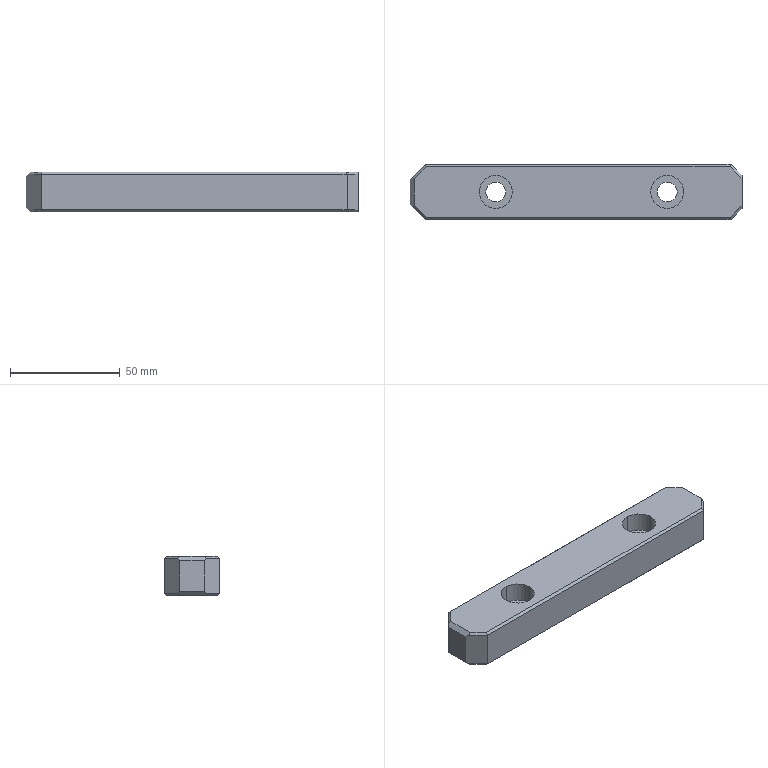Part | Creo | 1 solid | 34 faces | box 151 x 25 x 18 mm | volume 61935 mm3 | plane 26 | cylinder 8 | commonest cylinder face diameters 9 x4 15 x4
STEP:
#1=CARTESIAN_POINT('',(-121.,7.495,-46.5));
#2=VERTEX_POINT('',#1);
#3=CARTESIAN_POINT('',(-121.,7.495,-62.5));
#4=VERTEX_POINT('',#3);
#5=CARTESIAN_POINT('',(-121.,7.495,-46.5));
#6=DIRECTION('',(0.,0.,-1.));
#7=VECTOR('',#6,16.);
#8=LINE('',#5,#7);
#9=EDGE_CURVE('',#2,#4,#8,.T.);
#10=ORIENTED_EDGE('',*,*,#9,.T.);
#11=CARTESIAN_POINT('',(-121.,6.081,-63.5));
#12=VERTEX_POINT('',#11);
#13=CARTESIAN_POINT('',(-121.,6.081,-63.5));
#14=DIRECTION('',(0.,0.8165,0.5774));
#15=VECTOR('',#14,1.732);
#16=LINE('',#13,#15);
#17=EDGE_CURVE('',#12,#4,#16,.T.);
#18=ORIENTED_EDGE('',*,*,#17,.F.);
#19=CARTESIAN_POINT('',(-121.,-6.09,-63.5));
#20=VERTEX_POINT('',#19);
#21=CARTESIAN_POINT('',(-121.,6.081,-63.5));
#22=DIRECTION('',(0.,-1.,0.));
#23=VECTOR('',#22,12.172);
#24=LINE('',#21,#23);
#25=EDGE_CURVE('',#12,#20,#24,.T.);
#26=ORIENTED_EDGE('',*,*,#25,.T.);
#27=CARTESIAN_POINT('',(-121.,-7.505,-62.5));
#28=VERTEX_POINT('',#27);
#29=CARTESIAN_POINT('',(-121.,-7.505,-62.5));
#30=DIRECTION('',(0.,0.8165,-0.5774));
#31=VECTOR('',#30,1.732);
#32=LINE('',#29,#31);
#33=EDGE_CURVE('',#28,#20,#32,.T.);
#34=ORIENTED_EDGE('',*,*,#33,.F.);
#35=CARTESIAN_POINT('',(-121.,-7.505,-46.5));
#36=VERTEX_POINT('',#35);
#37=CARTESIAN_POINT('',(-121.,-7.505,-62.5));
#38=DIRECTION('',(0.,0.,1.));
#39=VECTOR('',#38,16.);
#40=LINE('',#37,#39);
#41=EDGE_CURVE('',#28,#36,#40,.T.);
#42=ORIENTED_EDGE('',*,*,#41,.T.);
#43=CARTESIAN_POINT('',(-121.,-6.09,-45.5));
#44=VERTEX_POINT('',#43);
#45=CARTESIAN_POINT('',(-121.,-6.09,-45.5));
#46=DIRECTION('',(0.,-0.8165,-0.5774));
#47=VECTOR('',#46,1.732);
#48=LINE('',#45,#47);
#49=EDGE_CURVE('',#44,#36,#48,.T.);
#50=ORIENTED_EDGE('',*,*,#49,.F.);
#51=CARTESIAN_POINT('',(-121.,6.081,-45.5));
#52=VERTEX_POINT('',#51);
#53=CARTESIAN_POINT('',(-121.,-6.09,-45.5));
#54=DIRECTION('',(0.,1.,0.));
#55=VECTOR('',#54,12.172);
#56=LINE('',#53,#55);
#57=EDGE_CURVE('',#44,#52,#56,.T.);
#58=ORIENTED_EDGE('',*,*,#57,.T.);
#59=CARTESIAN_POINT('',(-121.,7.495,-46.5));
#60=DIRECTION('',(0.,-0.8165,0.5774));
#61=VECTOR('',#60,1.732);
#62=LINE('',#59,#61);
#63=EDGE_CURVE('',#2,#52,#62,.T.);
#64=ORIENTED_EDGE('',*,*,#63,.F.);
#65=EDGE_LOOP('',(#10,#18,#26,#34,#42,#50,#58,#64));
#66=FACE_OUTER_BOUND('',#65,.F.);
#67=CARTESIAN_POINT('',(-121.,209.995,-11.));
#68=DIRECTION('',(-1.,0.,0.));
#69=DIRECTION('',(0.,-1.,0.));
#70=AXIS2_PLACEMENT_3D('',#67,#68,#69);
#71=PLANE('',#70);
#72=ADVANCED_FACE('',(#66),#71,.F.);
#73=CARTESIAN_POINT('',(-126.,12.495,-46.5));
#74=VERTEX_POINT('',#73);
#75=CARTESIAN_POINT('',(-126.,12.495,-62.5));
#76=VERTEX_POINT('',#75);
#77=CARTESIAN_POINT('',(-126.,12.495,-46.5));
#78=DIRECTION('',(0.,0.,-1.));
#79=VECTOR('',#78,16.);
#80=LINE('',#77,#79);
#81=EDGE_CURVE('',#74,#76,#80,.T.);
#82=ORIENTED_EDGE('',*,*,#81,.T.);
#83=CARTESIAN_POINT('',(-121.,7.495,-62.5));
#84=DIRECTION('',(-0.7071,0.7071,0.));
#85=VECTOR('',#84,7.071);
#86=LINE('',#83,#85);
#87=EDGE_CURVE('',#4,#76,#86,.T.);
#88=ORIENTED_EDGE('',*,*,#87,.F.);
#89=ORIENTED_EDGE('',*,*,#9,.F.);
#90=CARTESIAN_POINT('',(-121.,7.495,-46.5));
#91=DIRECTION('',(-0.7071,0.7071,0.));
#92=VECTOR('',#91,7.071);
#93=LINE('',#90,#92);
#94=EDGE_CURVE('',#2,#74,#93,.T.);
#95=ORIENTED_EDGE('',*,*,#94,.T.);
#96=EDGE_LOOP('',(#82,#88,#89,#95));
#97=FACE_OUTER_BOUND('',#96,.F.);
#98=CARTESIAN_POINT('',(-123.,9.495,-54.5));
#99=DIRECTION('',(0.7071,0.7071,0.));
#100=DIRECTION('',(0.,0.,-1.));
#101=AXIS2_PLACEMENT_3D('',#98,#99,#100);
#102=PLANE('',#101);
#103=ADVANCED_FACE('',(#97),#102,.T.);
#104=CARTESIAN_POINT('',(-265.,12.495,-62.5));
#105=VERTEX_POINT('',#104);
#106=CARTESIAN_POINT('',(-265.,12.495,-46.5));
#107=VERTEX_POINT('',#106);
#108=CARTESIAN_POINT('',(-265.,12.495,-62.5));
#109=DIRECTION('',(0.,0.,1.));
#110=VECTOR('',#109,16.);
#111=LINE('',#108,#110);
#112=EDGE_CURVE('',#105,#107,#111,.T.);
#113=ORIENTED_EDGE('',*,*,#112,.F.);
#114=CARTESIAN_POINT('',(-126.,12.495,-62.5));
#115=DIRECTION('',(-1.,0.,0.));
#116=VECTOR('',#115,139.);
#117=LINE('',#114,#116);
#118=EDGE_CURVE('',#76,#105,#117,.T.);
#119=ORIENTED_EDGE('',*,*,#118,.F.);
#120=ORIENTED_EDGE('',*,*,#81,.F.);
#121=CARTESIAN_POINT('',(-126.,12.495,-46.5));
#122=DIRECTION('',(-1.,0.,0.));
#123=VECTOR('',#122,139.);
#124=LINE('',#121,#123);
#125=EDGE_CURVE('',#74,#107,#124,.T.);
#126=ORIENTED_EDGE('',*,*,#125,.T.);
#127=EDGE_LOOP('',(#113,#119,#120,#126));
#128=FACE_OUTER_BOUND('',#127,.F.);
#129=CARTESIAN_POINT('',(-250.,12.495,-45.5));
#130=DIRECTION('',(0.,1.,0.));
#131=DIRECTION('',(0.,0.,1.));
#132=AXIS2_PLACEMENT_3D('',#129,#130,#131);
#133=PLANE('',#132);
#134=ADVANCED_FACE('',(#128),#133,.T.);
#135=CARTESIAN_POINT('',(-272.,5.495,-61.5));
#136=VERTEX_POINT('',#135);
#137=CARTESIAN_POINT('',(-272.,5.495,-47.5));
#138=VERTEX_POINT('',#137);
#139=CARTESIAN_POINT('',(-272.,5.495,-61.5));
#140=DIRECTION('',(0.,0.,1.));
#141=VECTOR('',#140,14.);
#142=LINE('',#139,#141);
#143=EDGE_CURVE('',#136,#138,#142,.T.);
#144=ORIENTED_EDGE('',*,*,#143,.F.);
#145=CARTESIAN_POINT('',(-271.,6.495,-62.5));
#146=VERTEX_POINT('',#145);
#147=CARTESIAN_POINT('',(-272.,5.495,-61.5));
#148=DIRECTION('',(0.5774,0.5774,-0.5774));
#149=VECTOR('',#148,1.732);
#150=LINE('',#147,#149);
#151=EDGE_CURVE('',#136,#146,#150,.T.);
#152=ORIENTED_EDGE('',*,*,#151,.T.);
#153=CARTESIAN_POINT('',(-265.,12.495,-62.5));
#154=DIRECTION('',(-0.7071,-0.7071,0.));
#155=VECTOR('',#154,8.485);
#156=LINE('',#153,#155);
#157=EDGE_CURVE('',#105,#146,#156,.T.);
#158=ORIENTED_EDGE('',*,*,#157,.F.);
#159=ORIENTED_EDGE('',*,*,#112,.T.);
#160=CARTESIAN_POINT('',(-271.,6.495,-46.5));
#161=VERTEX_POINT('',#160);
#162=CARTESIAN_POINT('',(-265.,12.495,-46.5));
#163=DIRECTION('',(-0.7071,-0.7071,0.));
#164=VECTOR('',#163,8.485);
#165=LINE('',#162,#164);
#166=EDGE_CURVE('',#107,#161,#165,.T.);
#167=ORIENTED_EDGE('',*,*,#166,.T.);
#168=CARTESIAN_POINT('',(-272.,5.495,-47.5));
#169=DIRECTION('',(0.5774,0.5774,0.5774));
#170=VECTOR('',#169,1.732);
#171=LINE('',#168,#170);
#172=EDGE_CURVE('',#138,#161,#171,.T.);
#173=ORIENTED_EDGE('',*,*,#172,.F.);
#174=EDGE_LOOP('',(#144,#152,#158,#159,#167,#173));
#175=FACE_OUTER_BOUND('',#174,.F.);
#176=CARTESIAN_POINT('',(-268.,9.495,-54.5));
#177=DIRECTION('',(-0.7071,0.7071,0.));
#178=DIRECTION('',(0.,0.,-1.));
#179=AXIS2_PLACEMENT_3D('',#176,#177,#178);
#180=PLANE('',#179);
#181=ADVANCED_FACE('',(#175),#180,.T.);
#182=CARTESIAN_POINT('',(-272.,-5.505,-47.5));
#183=VERTEX_POINT('',#182);
#184=CARTESIAN_POINT('',(-272.,-5.505,-61.5));
#185=VERTEX_POINT('',#184);
#186=CARTESIAN_POINT('',(-272.,-5.505,-47.5));
#187=DIRECTION('',(0.,0.,-1.));
#188=VECTOR('',#187,14.);
#189=LINE('',#186,#188);
#190=EDGE_CURVE('',#183,#185,#189,.T.);
#191=ORIENTED_EDGE('',*,*,#190,.T.);
#192=CARTESIAN_POINT('',(-272.,-5.505,-61.5));
#193=DIRECTION('',(0.,1.,0.));
#194=VECTOR('',#193,11.);
#195=LINE('',#192,#194);
#196=EDGE_CURVE('',#185,#136,#195,.T.);
#197=ORIENTED_EDGE('',*,*,#196,.T.);
#198=ORIENTED_EDGE('',*,*,#143,.T.);
#199=CARTESIAN_POINT('',(-272.,5.495,-47.5));
#200=DIRECTION('',(0.,-1.,0.));
#201=VECTOR('',#200,11.);
#202=LINE('',#199,#201);
#203=EDGE_CURVE('',#138,#183,#202,.T.);
#204=ORIENTED_EDGE('',*,*,#203,.T.);
#205=EDGE_LOOP('',(#191,#197,#198,#204));
#206=FACE_OUTER_BOUND('',#205,.F.);
#207=CARTESIAN_POINT('',(-272.,-3.005,-63.5));
#208=DIRECTION('',(1.,0.,0.));
#209=DIRECTION('',(0.,0.,-1.));
#210=AXIS2_PLACEMENT_3D('',#207,#208,#209);
#211=PLANE('',#210);
#212=ADVANCED_FACE('',(#206),#211,.F.);
#213=CARTESIAN_POINT('',(-265.,-12.505,-46.5));
#214=VERTEX_POINT('',#213);
#215=CARTESIAN_POINT('',(-265.,-12.505,-62.5));
#216=VERTEX_POINT('',#215);
#217=CARTESIAN_POINT('',(-265.,-12.505,-46.5));
#218=DIRECTION('',(0.,0.,-1.));
#219=VECTOR('',#218,16.);
#220=LINE('',#217,#219);
#221=EDGE_CURVE('',#214,#216,#220,.T.);
#222=ORIENTED_EDGE('',*,*,#221,.T.);
#223=CARTESIAN_POINT('',(-271.,-6.505,-62.5));
#224=VERTEX_POINT('',#223);
#225=CARTESIAN_POINT('',(-271.,-6.505,-62.5));
#226=DIRECTION('',(0.7071,-0.7071,0.));
#227=VECTOR('',#226,8.485);
#228=LINE('',#225,#227);
#229=EDGE_CURVE('',#224,#216,#228,.T.);
#230=ORIENTED_EDGE('',*,*,#229,.F.);
#231=CARTESIAN_POINT('',(-272.,-5.505,-61.5));
#232=DIRECTION('',(0.5774,-0.5774,-0.5774));
#233=VECTOR('',#232,1.732);
#234=LINE('',#231,#233);
#235=EDGE_CURVE('',#185,#224,#234,.T.);
#236=ORIENTED_EDGE('',*,*,#235,.F.);
#237=ORIENTED_EDGE('',*,*,#190,.F.);
#238=CARTESIAN_POINT('',(-271.,-6.505,-46.5));
#239=VERTEX_POINT('',#238);
#240=CARTESIAN_POINT('',(-272.,-5.505,-47.5));
#241=DIRECTION('',(0.5774,-0.5774,0.5774));
#242=VECTOR('',#241,1.732);
#243=LINE('',#240,#242);
#244=EDGE_CURVE('',#183,#239,#243,.T.);
#245=ORIENTED_EDGE('',*,*,#244,.T.);
#246=CARTESIAN_POINT('',(-271.,-6.505,-46.5));
#247=DIRECTION('',(0.7071,-0.7071,0.));
#248=VECTOR('',#247,8.485);
#249=LINE('',#246,#248);
#250=EDGE_CURVE('',#239,#214,#249,.T.);
#251=ORIENTED_EDGE('',*,*,#250,.T.);
#252=EDGE_LOOP('',(#222,#230,#236,#237,#245,#251));
#253=FACE_OUTER_BOUND('',#252,.F.);
#254=CARTESIAN_POINT('',(-268.,-9.505,-54.5));
#255=DIRECTION('',(-0.7071,-0.7071,0.));
#256=DIRECTION('',(0.,0.,-1.));
#257=AXIS2_PLACEMENT_3D('',#254,#255,#256);
#258=PLANE('',#257);
#259=ADVANCED_FACE('',(#253),#258,.T.);
#260=CARTESIAN_POINT('',(-126.,-12.505,-62.5));
#261=VERTEX_POINT('',#260);
#262=CARTESIAN_POINT('',(-126.,-12.505,-46.5));
#263=VERTEX_POINT('',#262);
#264=CARTESIAN_POINT('',(-126.,-12.505,-62.5));
#265=DIRECTION('',(0.,0.,1.));
#266=VECTOR('',#265,16.);
#267=LINE('',#264,#266);
#268=EDGE_CURVE('',#261,#263,#267,.T.);
#269=ORIENTED_EDGE('',*,*,#268,.F.);
#270=CARTESIAN_POINT('',(-126.,-12.505,-62.5));
#271=DIRECTION('',(-1.,0.,0.));
#272=VECTOR('',#271,139.);
#273=LINE('',#270,#272);
#274=EDGE_CURVE('',#261,#216,#273,.T.);
#275=ORIENTED_EDGE('',*,*,#274,.T.);
#276=ORIENTED_EDGE('',*,*,#221,.F.);
#277=CARTESIAN_POINT('',(-126.,-12.505,-46.5));
#278=DIRECTION('',(-1.,0.,0.));
#279=VECTOR('',#278,139.);
#280=LINE('',#277,#279);
#281=EDGE_CURVE('',#263,#214,#280,.T.);
#282=ORIENTED_EDGE('',*,*,#281,.F.);
#283=EDGE_LOOP('',(#269,#275,#276,#282));
#284=FACE_OUTER_BOUND('',#283,.F.);
#285=CARTESIAN_POINT('',(-250.,-12.505,-63.5));
#286=DIRECTION('',(0.,-1.,0.));
#287=DIRECTION('',(0.,0.,-1.));
#288=AXIS2_PLACEMENT_3D('',#285,#286,#287);
#289=PLANE('',#288);
#290=ADVANCED_FACE('',(#284),#289,.T.);
#291=ORIENTED_EDGE('',*,*,#41,.F.);
#292=CARTESIAN_POINT('',(-126.,-12.505,-62.5));
#293=DIRECTION('',(0.7071,0.7071,0.));
#294=VECTOR('',#293,7.071);
#295=LINE('',#292,#294);
#296=EDGE_CURVE('',#261,#28,#295,.T.);
#297=ORIENTED_EDGE('',*,*,#296,.F.);
#298=ORIENTED_EDGE('',*,*,#268,.T.);
#299=CARTESIAN_POINT('',(-126.,-12.505,-46.5));
#300=DIRECTION('',(0.7071,0.7071,0.));
#301=VECTOR('',#300,7.071);
#302=LINE('',#299,#301);
#303=EDGE_CURVE('',#263,#36,#302,.T.);
#304=ORIENTED_EDGE('',*,*,#303,.T.);
#305=EDGE_LOOP('',(#291,#297,#298,#304));
#306=FACE_OUTER_BOUND('',#305,.F.);
#307=CARTESIAN_POINT('',(-123.,-9.505,-54.5));
#308=DIRECTION('',(0.7071,-0.7071,0.));
#309=DIRECTION('',(0.,0.,-1.));
#310=AXIS2_PLACEMENT_3D('',#307,#308,#309);
#311=PLANE('',#310);
#312=ADVANCED_FACE('',(#306),#311,.T.);
#313=CARTESIAN_POINT('',(-126.414,-11.505,-63.5));
#314=VERTEX_POINT('',#313);
#315=CARTESIAN_POINT('',(-121.,-6.09,-63.5));
#316=DIRECTION('',(-0.7071,-0.7071,0.));
#317=VECTOR('',#316,7.657);
#318=LINE('',#315,#317);
#319=EDGE_CURVE('',#20,#314,#318,.T.);
#320=ORIENTED_EDGE('',*,*,#319,.T.);
#321=CARTESIAN_POINT('',(-126.414,-11.505,-63.5));
#322=DIRECTION('',(0.2811,-0.6786,0.6786));
#323=VECTOR('',#322,1.474);
#324=LINE('',#321,#323);
#325=EDGE_CURVE('',#314,#261,#324,.T.);
#326=ORIENTED_EDGE('',*,*,#325,.T.);
#327=ORIENTED_EDGE('',*,*,#296,.T.);
#328=ORIENTED_EDGE('',*,*,#33,.T.);
#329=EDGE_LOOP('',(#320,#326,#327,#328));
#330=FACE_OUTER_BOUND('',#329,.F.);
#331=CARTESIAN_POINT('',(-123.354,-9.151,-63.));
#332=DIRECTION('',(0.5,-0.5,-0.7071));
#333=DIRECTION('',(-0.5,0.5,-0.7071));
#334=AXIS2_PLACEMENT_3D('',#331,#332,#333);
#335=PLANE('',#334);
#336=ADVANCED_FACE('',(#330),#335,.T.);
#337=CARTESIAN_POINT('',(-264.586,-11.505,-63.5));
#338=VERTEX_POINT('',#337);
#339=CARTESIAN_POINT('',(-126.414,-11.505,-63.5));
#340=DIRECTION('',(-1.,0.,0.));
#341=VECTOR('',#340,138.172);
#342=LINE('',#339,#341);
#343=EDGE_CURVE('',#314,#338,#342,.T.);
#344=ORIENTED_EDGE('',*,*,#343,.F.);
#345=ORIENTED_EDGE('',*,*,#319,.F.);
#346=ORIENTED_EDGE('',*,*,#25,.F.);
#347=CARTESIAN_POINT('',(-126.414,11.495,-63.5));
#348=VERTEX_POINT('',#347);
#349=CARTESIAN_POINT('',(-126.414,11.495,-63.5));
#350=DIRECTION('',(0.7071,-0.7071,0.));
#351=VECTOR('',#350,7.657);
#352=LINE('',#349,#351);
#353=EDGE_CURVE('',#348,#12,#352,.T.);
#354=ORIENTED_EDGE('',*,*,#353,.F.);
#355=CARTESIAN_POINT('',(-264.586,11.495,-63.5));
#356=VERTEX_POINT('',#355);
#357=CARTESIAN_POINT('',(-126.414,11.495,-63.5));
#358=DIRECTION('',(-1.,0.,0.));
#359=VECTOR('',#358,138.172);
#360=LINE('',#357,#359);
#361=EDGE_CURVE('',#348,#356,#360,.T.);
#362=ORIENTED_EDGE('',*,*,#361,.T.);
#363=CARTESIAN_POINT('',(-270.,6.081,-63.5));
#364=VERTEX_POINT('',#363);
#365=CARTESIAN_POINT('',(-270.,6.081,-63.5));
#366=DIRECTION('',(0.7071,0.7071,0.));
#367=VECTOR('',#366,7.657);
#368=LINE('',#365,#367);
#369=EDGE_CURVE('',#364,#356,#368,.T.);
#370=ORIENTED_EDGE('',*,*,#369,.F.);
#371=CARTESIAN_POINT('',(-270.,-6.09,-63.5));
#372=VERTEX_POINT('',#371);
#373=CARTESIAN_POINT('',(-270.,-6.09,-63.5));
#374=DIRECTION('',(0.,1.,0.));
#375=VECTOR('',#374,12.172);
#376=LINE('',#373,#375);
#377=EDGE_CURVE('',#372,#364,#376,.T.);
#378=ORIENTED_EDGE('',*,*,#377,.F.);
#379=CARTESIAN_POINT('',(-264.586,-11.505,-63.5));
#380=DIRECTION('',(-0.7071,0.7071,0.));
#381=VECTOR('',#380,7.657);
#382=LINE('',#379,#381);
#383=EDGE_CURVE('',#338,#372,#382,.T.);
#384=ORIENTED_EDGE('',*,*,#383,.F.);
#385=EDGE_LOOP('',(#344,#345,#346,#354,#362,#370,#378,#384));
#386=FACE_OUTER_BOUND('',#385,.F.);
#387=CARTESIAN_POINT('',(-155.,4.495,-63.5));
#388=VERTEX_POINT('',#387);
#389=CARTESIAN_POINT('',(-155.,-4.505,-63.5));
#390=VERTEX_POINT('',#389);
#391=CARTESIAN_POINT('',(-155.,-0.004699,-63.5));
#392=DIRECTION('',(0.,0.,1.));
#393=DIRECTION('',(0.,1.,0.));
#394=AXIS2_PLACEMENT_3D('',#391,#392,#393);
#395=CIRCLE('',#394,4.5);
#396=EDGE_CURVE('',#388,#390,#395,.T.);
#397=ORIENTED_EDGE('',*,*,#396,.F.);
#398=CARTESIAN_POINT('',(-155.,-0.004699,-63.5));
#399=DIRECTION('',(0.,0.,1.));
#400=DIRECTION('',(0.,-1.,0.));
#401=AXIS2_PLACEMENT_3D('',#398,#399,#400);
#402=CIRCLE('',#401,4.5);
#403=EDGE_CURVE('',#390,#388,#402,.T.);
#404=ORIENTED_EDGE('',*,*,#403,.F.);
#405=EDGE_LOOP('',(#397,#404));
#406=FACE_BOUND('',#405,.F.);
#407=CARTESIAN_POINT('',(-233.,4.495,-63.5));
#408=VERTEX_POINT('',#407);
#409=CARTESIAN_POINT('',(-233.,-4.505,-63.5));
#410=VERTEX_POINT('',#409);
#411=CARTESIAN_POINT('',(-233.,-0.004699,-63.5));
#412=DIRECTION('',(0.,0.,1.));
#413=DIRECTION('',(0.,1.,0.));
#414=AXIS2_PLACEMENT_3D('',#411,#412,#413);
#415=CIRCLE('',#414,4.5);
#416=EDGE_CURVE('',#408,#410,#415,.T.);
#417=ORIENTED_EDGE('',*,*,#416,.F.);
#418=CARTESIAN_POINT('',(-233.,-0.004699,-63.5));
#419=DIRECTION('',(0.,0.,1.));
#420=DIRECTION('',(0.,-1.,0.));
#421=AXIS2_PLACEMENT_3D('',#418,#419,#420);
#422=CIRCLE('',#421,4.5);
#423=EDGE_CURVE('',#410,#408,#422,.T.);
#424=ORIENTED_EDGE('',*,*,#423,.F.);
#425=EDGE_LOOP('',(#417,#424));
#426=FACE_BOUND('',#425,.F.);
#427=CARTESIAN_POINT('',(-250.,12.495,-63.5));
#428=DIRECTION('',(0.,0.,-1.));
#429=DIRECTION('',(0.,1.,0.));
#430=AXIS2_PLACEMENT_3D('',#427,#428,#429);
#431=PLANE('',#430);
#432=ADVANCED_FACE('',(#386,#406,#426),#431,.T.);
#433=ORIENTED_EDGE('',*,*,#416,.T.);
#434=CARTESIAN_POINT('',(-233.,-4.505,-54.5));
#435=VERTEX_POINT('',#434);
#436=CARTESIAN_POINT('',(-233.,-4.505,-63.5));
#437=DIRECTION('',(0.,0.,1.));
#438=VECTOR('',#437,9.);
#439=LINE('',#436,#438);
#440=EDGE_CURVE('',#410,#435,#439,.T.);
#441=ORIENTED_EDGE('',*,*,#440,.T.);
#442=CARTESIAN_POINT('',(-233.,4.495,-54.5));
#443=VERTEX_POINT('',#442);
#444=CARTESIAN_POINT('',(-233.,-0.004699,-54.5));
#445=DIRECTION('',(0.,0.,-1.));
#446=DIRECTION('',(0.,-1.,0.));
#447=AXIS2_PLACEMENT_3D('',#444,#445,#446);
#448=CIRCLE('',#447,4.5);
#449=EDGE_CURVE('',#435,#443,#448,.T.);
#450=ORIENTED_EDGE('',*,*,#449,.T.);
#451=CARTESIAN_POINT('',(-233.,4.495,-63.5));
#452=DIRECTION('',(0.,0.,1.));
#453=VECTOR('',#452,9.);
#454=LINE('',#451,#453);
#455=EDGE_CURVE('',#408,#443,#454,.T.);
#456=ORIENTED_EDGE('',*,*,#455,.F.);
#457=EDGE_LOOP('',(#433,#441,#450,#456));
#458=FACE_OUTER_BOUND('',#457,.F.);
#459=CARTESIAN_POINT('',(-233.,-0.004699,-54.5));
#460=DIRECTION('',(0.,0.,1.));
#461=DIRECTION('',(0.,1.,0.));
#462=AXIS2_PLACEMENT_3D('',#459,#460,#461);
#463=CYLINDRICAL_SURFACE('',#462,4.5);
#464=ADVANCED_FACE('',(#458),#463,.F.);
#465=ORIENTED_EDGE('',*,*,#423,.T.);
#466=ORIENTED_EDGE('',*,*,#455,.T.);
#467=CARTESIAN_POINT('',(-233.,-0.004699,-54.5));
#468=DIRECTION('',(0.,0.,-1.));
#469=DIRECTION('',(0.,1.,0.));
#470=AXIS2_PLACEMENT_3D('',#467,#468,#469);
#471=CIRCLE('',#470,4.5);
#472=EDGE_CURVE('',#443,#435,#471,.T.);
#473=ORIENTED_EDGE('',*,*,#472,.T.);
#474=ORIENTED_EDGE('',*,*,#440,.F.);
#475=EDGE_LOOP('',(#465,#466,#473,#474));
#476=FACE_OUTER_BOUND('',#475,.F.);
#477=CARTESIAN_POINT('',(-233.,-0.004699,-54.5));
#478=DIRECTION('',(0.,0.,1.));
#479=DIRECTION('',(0.,1.,0.));
#480=AXIS2_PLACEMENT_3D('',#477,#478,#479);
#481=CYLINDRICAL_SURFACE('',#480,4.5);
#482=ADVANCED_FACE('',(#476),#481,.F.);
#483=CARTESIAN_POINT('',(-233.,-7.505,-54.5));
#484=VERTEX_POINT('',#483);
#485=CARTESIAN_POINT('',(-233.,7.495,-54.5));
#486=VERTEX_POINT('',#485);
#487=CARTESIAN_POINT('',(-233.,-0.004699,-54.5));
#488=DIRECTION('',(0.,0.,1.));
#489=DIRECTION('',(0.,-1.,0.));
#490=AXIS2_PLACEMENT_3D('',#487,#488,#489);
#491=CIRCLE('',#490,7.5);
#492=EDGE_CURVE('',#484,#486,#491,.T.);
#493=ORIENTED_EDGE('',*,*,#492,.F.);
#494=CARTESIAN_POINT('',(-233.,-0.004699,-54.5));
#495=DIRECTION('',(0.,0.,1.));
#496=DIRECTION('',(0.,1.,0.));
#497=AXIS2_PLACEMENT_3D('',#494,#495,#496);
#498=CIRCLE('',#497,7.5);
#499=EDGE_CURVE('',#486,#484,#498,.T.);
#500=ORIENTED_EDGE('',*,*,#499,.F.);
#501=EDGE_LOOP('',(#493,#500));
#502=FACE_OUTER_BOUND('',#501,.F.);
#503=ORIENTED_EDGE('',*,*,#472,.F.);
#504=ORIENTED_EDGE('',*,*,#449,.F.);
#505=EDGE_LOOP('',(#503,#504));
#506=FACE_BOUND('',#505,.F.);
#507=CARTESIAN_POINT('',(-233.,-0.004699,-54.5));
#508=DIRECTION('',(0.,0.,-1.));
#509=DIRECTION('',(0.,1.,0.));
#510=AXIS2_PLACEMENT_3D('',#507,#508,#509);
#511=PLANE('',#510);
#512=ADVANCED_FACE('',(#502,#506),#511,.F.);
#513=CARTESIAN_POINT('',(-233.,7.495,-45.5));
#514=VERTEX_POINT('',#513);
#515=CARTESIAN_POINT('',(-233.,-7.505,-45.5));
#516=VERTEX_POINT('',#515);
#517=CARTESIAN_POINT('',(-233.,-0.004699,-45.5));
#518=DIRECTION('',(0.,0.,-1.));
#519=DIRECTION('',(0.,1.,0.));
#520=AXIS2_PLACEMENT_3D('',#517,#518,#519);
#521=CIRCLE('',#520,7.5);
#522=EDGE_CURVE('',#514,#516,#521,.T.);
#523=ORIENTED_EDGE('',*,*,#522,.T.);
#524=CARTESIAN_POINT('',(-233.,-7.505,-45.5));
#525=DIRECTION('',(0.,0.,-1.));
#526=VECTOR('',#525,9.);
#527=LINE('',#524,#526);
#528=EDGE_CURVE('',#516,#484,#527,.T.);
#529=ORIENTED_EDGE('',*,*,#528,.T.);
#530=ORIENTED_EDGE('',*,*,#492,.T.);
#531=CARTESIAN_POINT('',(-233.,7.495,-45.5));
#532=DIRECTION('',(0.,0.,-1.));
#533=VECTOR('',#532,9.);
#534=LINE('',#531,#533);
#535=EDGE_CURVE('',#514,#486,#534,.T.);
#536=ORIENTED_EDGE('',*,*,#535,.F.);
#537=EDGE_LOOP('',(#523,#529,#530,#536));
#538=FACE_OUTER_BOUND('',#537,.F.);
#539=CARTESIAN_POINT('',(-233.,-0.004699,-45.05));
#540=DIRECTION('',(0.,0.,-1.));
#541=DIRECTION('',(0.,1.,0.));
#542=AXIS2_PLACEMENT_3D('',#539,#540,#541);
#543=CYLINDRICAL_SURFACE('',#542,7.5);
#544=ADVANCED_FACE('',(#538),#543,.F.);
#545=CARTESIAN_POINT('',(-270.,6.081,-45.5));
#546=VERTEX_POINT('',#545);
#547=CARTESIAN_POINT('',(-264.586,11.495,-45.5));
#548=VERTEX_POINT('',#547);
#549=CARTESIAN_POINT('',(-270.,6.081,-45.5));
#550=DIRECTION('',(0.7071,0.7071,0.));
#551=VECTOR('',#550,7.657);
#552=LINE('',#549,#551);
#553=EDGE_CURVE('',#546,#548,#552,.T.);
#554=ORIENTED_EDGE('',*,*,#553,.T.);
#555=CARTESIAN_POINT('',(-126.414,11.495,-45.5));
#556=VERTEX_POINT('',#555);
#557=CARTESIAN_POINT('',(-126.414,11.495,-45.5));
#558=DIRECTION('',(-1.,0.,0.));
#559=VECTOR('',#558,138.172);
#560=LINE('',#557,#559);
#561=EDGE_CURVE('',#556,#548,#560,.T.);
#562=ORIENTED_EDGE('',*,*,#561,.F.);
#563=CARTESIAN_POINT('',(-126.414,11.495,-45.5));
#564=DIRECTION('',(0.7071,-0.7071,0.));
#565=VECTOR('',#564,7.657);
#566=LINE('',#563,#565);
#567=EDGE_CURVE('',#556,#52,#566,.T.);
#568=ORIENTED_EDGE('',*,*,#567,.T.);
#569=ORIENTED_EDGE('',*,*,#57,.F.);
#570=CARTESIAN_POINT('',(-126.414,-11.505,-45.5));
#571=VERTEX_POINT('',#570);
#572=CARTESIAN_POINT('',(-121.,-6.09,-45.5));
#573=DIRECTION('',(-0.7071,-0.7071,0.));
#574=VECTOR('',#573,7.657);
#575=LINE('',#572,#574);
#576=EDGE_CURVE('',#44,#571,#575,.T.);
#577=ORIENTED_EDGE('',*,*,#576,.T.);
#578=CARTESIAN_POINT('',(-264.586,-11.505,-45.5));
#579=VERTEX_POINT('',#578);
#580=CARTESIAN_POINT('',(-126.414,-11.505,-45.5));
#581=DIRECTION('',(-1.,0.,0.));
#582=VECTOR('',#581,138.172);
#583=LINE('',#580,#582);
#584=EDGE_CURVE('',#571,#579,#583,.T.);
#585=ORIENTED_EDGE('',*,*,#584,.T.);
#586=CARTESIAN_POINT('',(-270.,-6.09,-45.5));
#587=VERTEX_POINT('',#586);
#588=CARTESIAN_POINT('',(-264.586,-11.505,-45.5));
#589=DIRECTION('',(-0.7071,0.7071,0.));
#590=VECTOR('',#589,7.657);
#591=LINE('',#588,#590);
#592=EDGE_CURVE('',#579,#587,#591,.T.);
#593=ORIENTED_EDGE('',*,*,#592,.T.);
#594=CARTESIAN_POINT('',(-270.,6.081,-45.5));
#595=DIRECTION('',(0.,-1.,0.));
#596=VECTOR('',#595,12.172);
#597=LINE('',#594,#596);
#598=EDGE_CURVE('',#546,#587,#597,.T.);
#599=ORIENTED_EDGE('',*,*,#598,.F.);
#600=EDGE_LOOP('',(#554,#562,#568,#569,#577,#585,#593,#599));
#601=FACE_OUTER_BOUND('',#600,.F.);
#602=CARTESIAN_POINT('',(-155.,7.495,-45.5));
#603=VERTEX_POINT('',#602);
#604=CARTESIAN_POINT('',(-155.,-7.505,-45.5));
#605=VERTEX_POINT('',#604);
#606=CARTESIAN_POINT('',(-155.,-0.004699,-45.5));
#607=DIRECTION('',(0.,0.,-1.));
#608=DIRECTION('',(0.,1.,0.));
#609=AXIS2_PLACEMENT_3D('',#606,#607,#608);
#610=CIRCLE('',#609,7.5);
#611=EDGE_CURVE('',#603,#605,#610,.T.);
#612=ORIENTED_EDGE('',*,*,#611,.F.);
#613=CARTESIAN_POINT('',(-155.,-0.004699,-45.5));
#614=DIRECTION('',(0.,0.,-1.));
#615=DIRECTION('',(0.,-1.,0.));
#616=AXIS2_PLACEMENT_3D('',#613,#614,#615);
#617=CIRCLE('',#616,7.5);
#618=EDGE_CURVE('',#605,#603,#617,.T.);
#619=ORIENTED_EDGE('',*,*,#618,.F.);
#620=EDGE_LOOP('',(#612,#619));
#621=FACE_BOUND('',#620,.F.);
#622=ORIENTED_EDGE('',*,*,#522,.F.);
#623=CARTESIAN_POINT('',(-233.,-0.004699,-45.5));
#624=DIRECTION('',(0.,0.,-1.));
#625=DIRECTION('',(0.,-1.,0.));
#626=AXIS2_PLACEMENT_3D('',#623,#624,#625);
#627=CIRCLE('',#626,7.5);
#628=EDGE_CURVE('',#516,#514,#627,.T.);
#629=ORIENTED_EDGE('',*,*,#628,.F.);
#630=EDGE_LOOP('',(#622,#629));
#631=FACE_BOUND('',#630,.F.);
#632=CARTESIAN_POINT('',(-250.,-12.505,-45.5));
#633=DIRECTION('',(0.,0.,1.));
#634=DIRECTION('',(0.,-1.,0.));
#635=AXIS2_PLACEMENT_3D('',#632,#633,#634);
#636=PLANE('',#635);
#637=ADVANCED_FACE('',(#601,#621,#631),#636,.T.);
#638=ORIENTED_EDGE('',*,*,#628,.T.);
#639=ORIENTED_EDGE('',*,*,#535,.T.);
#640=ORIENTED_EDGE('',*,*,#499,.T.);
#641=ORIENTED_EDGE('',*,*,#528,.F.);
#642=EDGE_LOOP('',(#638,#639,#640,#641));
#643=FACE_OUTER_BOUND('',#642,.F.);
#644=CARTESIAN_POINT('',(-233.,-0.004699,-45.05));
#645=DIRECTION('',(0.,0.,-1.));
#646=DIRECTION('',(0.,1.,0.));
#647=AXIS2_PLACEMENT_3D('',#644,#645,#646);
#648=CYLINDRICAL_SURFACE('',#647,7.5);
#649=ADVANCED_FACE('',(#643),#648,.F.);
#650=ORIENTED_EDGE('',*,*,#611,.T.);
#651=CARTESIAN_POINT('',(-155.,-7.505,-54.5));
#652=VERTEX_POINT('',#651);
#653=CARTESIAN_POINT('',(-155.,-7.505,-45.5));
#654=DIRECTION('',(0.,0.,-1.));
#655=VECTOR('',#654,9.);
#656=LINE('',#653,#655);
#657=EDGE_CURVE('',#605,#652,#656,.T.);
#658=ORIENTED_EDGE('',*,*,#657,.T.);
#659=CARTESIAN_POINT('',(-155.,7.495,-54.5));
#660=VERTEX_POINT('',#659);
#661=CARTESIAN_POINT('',(-155.,-0.004699,-54.5));
#662=DIRECTION('',(0.,0.,1.));
#663=DIRECTION('',(0.,-1.,0.));
#664=AXIS2_PLACEMENT_3D('',#661,#662,#663);
#665=CIRCLE('',#664,7.5);
#666=EDGE_CURVE('',#652,#660,#665,.T.);
#667=ORIENTED_EDGE('',*,*,#666,.T.);
#668=CARTESIAN_POINT('',(-155.,7.495,-45.5));
#669=DIRECTION('',(0.,0.,-1.));
#670=VECTOR('',#669,9.);
#671=LINE('',#668,#670);
#672=EDGE_CURVE('',#603,#660,#671,.T.);
#673=ORIENTED_EDGE('',*,*,#672,.F.);
#674=EDGE_LOOP('',(#650,#658,#667,#673));
#675=FACE_OUTER_BOUND('',#674,.F.);
#676=CARTESIAN_POINT('',(-155.,-0.004699,-45.05));
#677=DIRECTION('',(0.,0.,-1.));
#678=DIRECTION('',(0.,1.,0.));
#679=AXIS2_PLACEMENT_3D('',#676,#677,#678);
#680=CYLINDRICAL_SURFACE('',#679,7.5);
#681=ADVANCED_FACE('',(#675),#680,.F.);
#682=ORIENTED_EDGE('',*,*,#618,.T.);
#683=ORIENTED_EDGE('',*,*,#672,.T.);
#684=CARTESIAN_POINT('',(-155.,-0.004699,-54.5));
#685=DIRECTION('',(0.,0.,1.));
#686=DIRECTION('',(0.,1.,0.));
#687=AXIS2_PLACEMENT_3D('',#684,#685,#686);
#688=CIRCLE('',#687,7.5);
#689=EDGE_CURVE('',#660,#652,#688,.T.);
#690=ORIENTED_EDGE('',*,*,#689,.T.);
#691=ORIENTED_EDGE('',*,*,#657,.F.);
#692=EDGE_LOOP('',(#682,#683,#690,#691));
#693=FACE_OUTER_BOUND('',#692,.F.);
#694=CARTESIAN_POINT('',(-155.,-0.004699,-45.05));
#695=DIRECTION('',(0.,0.,-1.));
#696=DIRECTION('',(0.,1.,0.));
#697=AXIS2_PLACEMENT_3D('',#694,#695,#696);
#698=CYLINDRICAL_SURFACE('',#697,7.5);
#699=ADVANCED_FACE('',(#693),#698,.F.);
#700=ORIENTED_EDGE('',*,*,#666,.F.);
#701=ORIENTED_EDGE('',*,*,#689,.F.);
#702=EDGE_LOOP('',(#700,#701));
#703=FACE_OUTER_BOUND('',#702,.F.);
#704=CARTESIAN_POINT('',(-155.,4.495,-54.5));
#705=VERTEX_POINT('',#704);
#706=CARTESIAN_POINT('',(-155.,-4.505,-54.5));
#707=VERTEX_POINT('',#706);
#708=CARTESIAN_POINT('',(-155.,-0.004699,-54.5));
#709=DIRECTION('',(0.,0.,-1.));
#710=DIRECTION('',(0.,1.,0.));
#711=AXIS2_PLACEMENT_3D('',#708,#709,#710);
#712=CIRCLE('',#711,4.5);
#713=EDGE_CURVE('',#705,#707,#712,.T.);
#714=ORIENTED_EDGE('',*,*,#713,.F.);
#715=CARTESIAN_POINT('',(-155.,-0.004699,-54.5));
#716=DIRECTION('',(0.,0.,-1.));
#717=DIRECTION('',(0.,-1.,0.));
#718=AXIS2_PLACEMENT_3D('',#715,#716,#717);
#719=CIRCLE('',#718,4.5);
#720=EDGE_CURVE('',#707,#705,#719,.T.);
#721=ORIENTED_EDGE('',*,*,#720,.F.);
#722=EDGE_LOOP('',(#714,#721));
#723=FACE_BOUND('',#722,.F.);
#724=CARTESIAN_POINT('',(-155.,-0.004699,-54.5));
#725=DIRECTION('',(0.,0.,-1.));
#726=DIRECTION('',(0.,1.,0.));
#727=AXIS2_PLACEMENT_3D('',#724,#725,#726);
#728=PLANE('',#727);
#729=ADVANCED_FACE('',(#703,#723),#728,.F.);
#730=ORIENTED_EDGE('',*,*,#403,.T.);
#731=CARTESIAN_POINT('',(-155.,4.495,-63.5));
#732=DIRECTION('',(0.,0.,1.));
#733=VECTOR('',#732,9.);
#734=LINE('',#731,#733);
#735=EDGE_CURVE('',#388,#705,#734,.T.);
#736=ORIENTED_EDGE('',*,*,#735,.T.);
#737=ORIENTED_EDGE('',*,*,#713,.T.);
#738=CARTESIAN_POINT('',(-155.,-4.505,-63.5));
#739=DIRECTION('',(0.,0.,1.));
#740=VECTOR('',#739,9.);
#741=LINE('',#738,#740);
#742=EDGE_CURVE('',#390,#707,#741,.T.);
#743=ORIENTED_EDGE('',*,*,#742,.F.);
#744=EDGE_LOOP('',(#730,#736,#737,#743));
#745=FACE_OUTER_BOUND('',#744,.F.);
#746=CARTESIAN_POINT('',(-155.,-0.004699,-54.5));
#747=DIRECTION('',(0.,0.,1.));
#748=DIRECTION('',(0.,1.,0.));
#749=AXIS2_PLACEMENT_3D('',#746,#747,#748);
#750=CYLINDRICAL_SURFACE('',#749,4.5);
#751=ADVANCED_FACE('',(#745),#750,.F.);
#752=ORIENTED_EDGE('',*,*,#396,.T.);
#753=ORIENTED_EDGE('',*,*,#742,.T.);
#754=ORIENTED_EDGE('',*,*,#720,.T.);
#755=ORIENTED_EDGE('',*,*,#735,.F.);
#756=EDGE_LOOP('',(#752,#753,#754,#755));
#757=FACE_OUTER_BOUND('',#756,.F.);
#758=CARTESIAN_POINT('',(-155.,-0.004699,-54.5));
#759=DIRECTION('',(0.,0.,1.));
#760=DIRECTION('',(0.,1.,0.));
#761=AXIS2_PLACEMENT_3D('',#758,#759,#760);
#762=CYLINDRICAL_SURFACE('',#761,4.5);
#763=ADVANCED_FACE('',(#757),#762,.F.);
#764=ORIENTED_EDGE('',*,*,#553,.F.);
#765=CARTESIAN_POINT('',(-270.,6.081,-45.5));
#766=DIRECTION('',(-0.6786,0.2811,-0.6786));
#767=VECTOR('',#766,1.474);
#768=LINE('',#765,#767);
#769=EDGE_CURVE('',#546,#161,#768,.T.);
#770=ORIENTED_EDGE('',*,*,#769,.T.);
#771=ORIENTED_EDGE('',*,*,#166,.F.);
#772=CARTESIAN_POINT('',(-265.,12.495,-46.5));
#773=DIRECTION('',(0.2811,-0.6786,0.6786));
#774=VECTOR('',#773,1.474);
#775=LINE('',#772,#774);
#776=EDGE_CURVE('',#107,#548,#775,.T.);
#777=ORIENTED_EDGE('',*,*,#776,.T.);
#778=EDGE_LOOP('',(#764,#770,#771,#777));
#779=FACE_OUTER_BOUND('',#778,.F.);
#780=CARTESIAN_POINT('',(-267.646,9.142,-46.));
#781=DIRECTION('',(-0.5,0.5,0.7071));
#782=DIRECTION('',(-0.866,-0.2887,-0.4082));
#783=AXIS2_PLACEMENT_3D('',#780,#781,#782);
#784=PLANE('',#783);
#785=ADVANCED_FACE('',(#779),#784,.T.);
#786=ORIENTED_EDGE('',*,*,#598,.T.);
#787=CARTESIAN_POINT('',(-270.,-6.09,-45.5));
#788=DIRECTION('',(-0.6786,-0.2811,-0.6786));
#789=VECTOR('',#788,1.474);
#790=LINE('',#787,#789);
#791=EDGE_CURVE('',#587,#239,#790,.T.);
#792=ORIENTED_EDGE('',*,*,#791,.T.);
#793=ORIENTED_EDGE('',*,*,#244,.F.);
#794=ORIENTED_EDGE('',*,*,#203,.F.);
#795=ORIENTED_EDGE('',*,*,#172,.T.);
#796=ORIENTED_EDGE('',*,*,#769,.F.);
#797=EDGE_LOOP('',(#786,#792,#793,#794,#795,#796));
#798=FACE_OUTER_BOUND('',#797,.F.);
#799=CARTESIAN_POINT('',(-270.5,-0.004699,-46.));
#800=DIRECTION('',(-0.7071,0.,0.7071));
#801=DIRECTION('',(0.,-1.,0.));
#802=AXIS2_PLACEMENT_3D('',#799,#800,#801);
#803=PLANE('',#802);
#804=ADVANCED_FACE('',(#798),#803,.T.);
#805=ORIENTED_EDGE('',*,*,#592,.F.);
#806=CARTESIAN_POINT('',(-264.586,-11.505,-45.5));
#807=DIRECTION('',(-0.2811,-0.6786,-0.6786));
#808=VECTOR('',#807,1.474);
#809=LINE('',#806,#808);
#810=EDGE_CURVE('',#579,#214,#809,.T.);
#811=ORIENTED_EDGE('',*,*,#810,.T.);
#812=ORIENTED_EDGE('',*,*,#250,.F.);
#813=ORIENTED_EDGE('',*,*,#791,.F.);
#814=EDGE_LOOP('',(#805,#811,#812,#813));
#815=FACE_OUTER_BOUND('',#814,.F.);
#816=CARTESIAN_POINT('',(-267.646,-9.151,-46.));
#817=DIRECTION('',(-0.5,-0.5,0.7071));
#818=DIRECTION('',(-0.866,0.2887,-0.4082));
#819=AXIS2_PLACEMENT_3D('',#816,#817,#818);
#820=PLANE('',#819);
#821=ADVANCED_FACE('',(#815),#820,.T.);
#822=CARTESIAN_POINT('',(-126.,-12.505,-46.5));
#823=DIRECTION('',(-0.2811,0.6786,0.6786));
#824=VECTOR('',#823,1.474);
#825=LINE('',#822,#824);
#826=EDGE_CURVE('',#263,#571,#825,.T.);
#827=ORIENTED_EDGE('',*,*,#826,.F.);
#828=ORIENTED_EDGE('',*,*,#281,.T.);
#829=ORIENTED_EDGE('',*,*,#810,.F.);
#830=ORIENTED_EDGE('',*,*,#584,.F.);
#831=EDGE_LOOP('',(#827,#828,#829,#830));
#832=FACE_OUTER_BOUND('',#831,.F.);
#833=CARTESIAN_POINT('',(-167.5,-12.005,-46.));
#834=DIRECTION('',(0.,-0.7071,0.7071));
#835=DIRECTION('',(-1.,0.,0.));
#836=AXIS2_PLACEMENT_3D('',#833,#834,#835);
#837=PLANE('',#836);
#838=ADVANCED_FACE('',(#832),#837,.T.);
#839=ORIENTED_EDGE('',*,*,#576,.F.);
#840=ORIENTED_EDGE('',*,*,#49,.T.);
#841=ORIENTED_EDGE('',*,*,#303,.F.);
#842=ORIENTED_EDGE('',*,*,#826,.T.);
#843=EDGE_LOOP('',(#839,#840,#841,#842));
#844=FACE_OUTER_BOUND('',#843,.F.);
#845=CARTESIAN_POINT('',(-123.354,-9.151,-46.));
#846=DIRECTION('',(0.5,-0.5,0.7071));
#847=DIRECTION('',(-0.866,-0.2887,0.4082));
#848=AXIS2_PLACEMENT_3D('',#845,#846,#847);
#849=PLANE('',#848);
#850=ADVANCED_FACE('',(#844),#849,.T.);
#851=CARTESIAN_POINT('',(-126.414,11.495,-45.5));
#852=DIRECTION('',(0.2811,0.6786,-0.6786));
#853=VECTOR('',#852,1.474);
#854=LINE('',#851,#853);
#855=EDGE_CURVE('',#556,#74,#854,.T.);
#856=ORIENTED_EDGE('',*,*,#855,.F.);
#857=ORIENTED_EDGE('',*,*,#561,.T.);
#858=ORIENTED_EDGE('',*,*,#776,.F.);
#859=ORIENTED_EDGE('',*,*,#125,.F.);
#860=EDGE_LOOP('',(#856,#857,#858,#859));
#861=FACE_OUTER_BOUND('',#860,.F.);
#862=CARTESIAN_POINT('',(-167.5,11.995,-46.));
#863=DIRECTION('',(0.,0.7071,0.7071));
#864=DIRECTION('',(-1.,0.,0.));
#865=AXIS2_PLACEMENT_3D('',#862,#863,#864);
#866=PLANE('',#865);
#867=ADVANCED_FACE('',(#861),#866,.T.);
#868=ORIENTED_EDGE('',*,*,#94,.F.);
#869=ORIENTED_EDGE('',*,*,#63,.T.);
#870=ORIENTED_EDGE('',*,*,#567,.F.);
#871=ORIENTED_EDGE('',*,*,#855,.T.);
#872=EDGE_LOOP('',(#868,#869,#870,#871));
#873=FACE_OUTER_BOUND('',#872,.F.);
#874=CARTESIAN_POINT('',(-123.354,9.142,-46.));
#875=DIRECTION('',(0.5,0.5,0.7071));
#876=DIRECTION('',(-0.866,0.2887,0.4082));
#877=AXIS2_PLACEMENT_3D('',#874,#875,#876);
#878=PLANE('',#877);
#879=ADVANCED_FACE('',(#873),#878,.T.);
#880=ORIENTED_EDGE('',*,*,#325,.F.);
#881=ORIENTED_EDGE('',*,*,#343,.T.);
#882=CARTESIAN_POINT('',(-264.586,-11.505,-63.5));
#883=DIRECTION('',(-0.2811,-0.6786,0.6786));
#884=VECTOR('',#883,1.474);
#885=LINE('',#882,#884);
#886=EDGE_CURVE('',#338,#216,#885,.T.);
#887=ORIENTED_EDGE('',*,*,#886,.T.);
#888=ORIENTED_EDGE('',*,*,#274,.F.);
#889=EDGE_LOOP('',(#880,#881,#887,#888));
#890=FACE_OUTER_BOUND('',#889,.F.);
#891=CARTESIAN_POINT('',(-167.5,-12.005,-63.));
#892=DIRECTION('',(0.,-0.7071,-0.7071));
#893=DIRECTION('',(0.,-0.7071,0.7071));
#894=AXIS2_PLACEMENT_3D('',#891,#892,#893);
#895=PLANE('',#894);
#896=ADVANCED_FACE('',(#890),#895,.T.);
#897=CARTESIAN_POINT('',(-270.,-6.09,-63.5));
#898=DIRECTION('',(-0.6786,-0.2811,0.6786));
#899=VECTOR('',#898,1.474);
#900=LINE('',#897,#899);
#901=EDGE_CURVE('',#372,#224,#900,.T.);
#902=ORIENTED_EDGE('',*,*,#901,.T.);
#903=ORIENTED_EDGE('',*,*,#229,.T.);
#904=ORIENTED_EDGE('',*,*,#886,.F.);
#905=ORIENTED_EDGE('',*,*,#383,.T.);
#906=EDGE_LOOP('',(#902,#903,#904,#905));
#907=FACE_OUTER_BOUND('',#906,.F.);
#908=CARTESIAN_POINT('',(-267.646,-9.151,-63.));
#909=DIRECTION('',(-0.5,-0.5,-0.7071));
#910=DIRECTION('',(0.5,0.5,-0.7071));
#911=AXIS2_PLACEMENT_3D('',#908,#909,#910);
#912=PLANE('',#911);
#913=ADVANCED_FACE('',(#907),#912,.T.);
#914=ORIENTED_EDGE('',*,*,#901,.F.);
#915=ORIENTED_EDGE('',*,*,#377,.T.);
#916=CARTESIAN_POINT('',(-270.,6.081,-63.5));
#917=DIRECTION('',(-0.6786,0.2811,0.6786));
#918=VECTOR('',#917,1.474);
#919=LINE('',#916,#918);
#920=EDGE_CURVE('',#364,#146,#919,.T.);
#921=ORIENTED_EDGE('',*,*,#920,.T.);
#922=ORIENTED_EDGE('',*,*,#151,.F.);
#923=ORIENTED_EDGE('',*,*,#196,.F.);
#924=ORIENTED_EDGE('',*,*,#235,.T.);
#925=EDGE_LOOP('',(#914,#915,#921,#922,#923,#924));
#926=FACE_OUTER_BOUND('',#925,.F.);
#927=CARTESIAN_POINT('',(-270.5,-0.004699,-63.));
#928=DIRECTION('',(-0.7071,0.,-0.7071));
#929=DIRECTION('',(-0.7071,0.,0.7071));
#930=AXIS2_PLACEMENT_3D('',#927,#928,#929);
#931=PLANE('',#930);
#932=ADVANCED_FACE('',(#926),#931,.T.);
#933=ORIENTED_EDGE('',*,*,#920,.F.);
#934=ORIENTED_EDGE('',*,*,#369,.T.);
#935=CARTESIAN_POINT('',(-264.586,11.495,-63.5));
#936=DIRECTION('',(-0.2811,0.6786,0.6786));
#937=VECTOR('',#936,1.474);
#938=LINE('',#935,#937);
#939=EDGE_CURVE('',#356,#105,#938,.T.);
#940=ORIENTED_EDGE('',*,*,#939,.T.);
#941=ORIENTED_EDGE('',*,*,#157,.T.);
#942=EDGE_LOOP('',(#933,#934,#940,#941));
#943=FACE_OUTER_BOUND('',#942,.F.);
#944=CARTESIAN_POINT('',(-267.646,9.142,-63.));
#945=DIRECTION('',(-0.5,0.5,-0.7071));
#946=DIRECTION('',(0.5,-0.5,-0.7071));
#947=AXIS2_PLACEMENT_3D('',#944,#945,#946);
#948=PLANE('',#947);
#949=ADVANCED_FACE('',(#943),#948,.T.);
#950=CARTESIAN_POINT('',(-126.,12.495,-62.5));
#951=DIRECTION('',(-0.2811,-0.6786,-0.6786));
#952=VECTOR('',#951,1.474);
#953=LINE('',#950,#952);
#954=EDGE_CURVE('',#76,#348,#953,.T.);
#955=ORIENTED_EDGE('',*,*,#954,.F.);
#956=ORIENTED_EDGE('',*,*,#118,.T.);
#957=ORIENTED_EDGE('',*,*,#939,.F.);
#958=ORIENTED_EDGE('',*,*,#361,.F.);
#959=EDGE_LOOP('',(#955,#956,#957,#958));
#960=FACE_OUTER_BOUND('',#959,.F.);
#961=CARTESIAN_POINT('',(-167.5,11.995,-63.));
#962=DIRECTION('',(0.,0.7071,-0.7071));
#963=DIRECTION('',(0.,-0.7071,-0.7071));
#964=AXIS2_PLACEMENT_3D('',#961,#962,#963);
#965=PLANE('',#964);
#966=ADVANCED_FACE('',(#960),#965,.T.);
#967=ORIENTED_EDGE('',*,*,#17,.T.);
#968=ORIENTED_EDGE('',*,*,#87,.T.);
#969=ORIENTED_EDGE('',*,*,#954,.T.);
#970=ORIENTED_EDGE('',*,*,#353,.T.);
#971=EDGE_LOOP('',(#967,#968,#969,#970));
#972=FACE_OUTER_BOUND('',#971,.F.);
#973=CARTESIAN_POINT('',(-123.354,9.142,-63.));
#974=DIRECTION('',(0.5,0.5,-0.7071));
#975=DIRECTION('',(-0.5,-0.5,-0.7071));
#976=AXIS2_PLACEMENT_3D('',#973,#974,#975);
#977=PLANE('',#976);
#978=ADVANCED_FACE('',(#972),#977,.T.);
#979=CLOSED_SHELL('',(#72,#103,#134,#181,#212,#259,#290,#312,#336,#432,#464,#482,#512,#544,#637,#649,#681,#699,#729,#751,#763,#785,#804,#821,#838,#850,#867,#879,#896,#913,#932,#949,#966,#978));
#980=MANIFOLD_SOLID_BREP('',#979);
#981=(LENGTH_UNIT()NAMED_UNIT(*)SI_UNIT(.MILLI.,.METRE.));
#982=UNCERTAINTY_MEASURE_WITH_UNIT(LENGTH_MEASURE(0.01552),#981,'','');
#983=(NAMED_UNIT(*)PLANE_ANGLE_UNIT()SI_UNIT($,.RADIAN.));
#984=PLANE_ANGLE_MEASURE_WITH_UNIT(PLANE_ANGLE_MEASURE(0.01745),#983);
#985=(CONVERSION_BASED_UNIT('DEGREE',#984)NAMED_UNIT(*)PLANE_ANGLE_UNIT());
#986=(NAMED_UNIT(*)SI_UNIT($,.STERADIAN.)SOLID_ANGLE_UNIT());
#987=(GEOMETRIC_REPRESENTATION_CONTEXT(3)GLOBAL_UNCERTAINTY_ASSIGNED_CONTEXT((#982))GLOBAL_UNIT_ASSIGNED_CONTEXT((#981,#985,#986))REPRESENTATION_CONTEXT('',''));
#988=ADVANCED_BREP_SHAPE_REPRESENTATION('',(#980),#987);